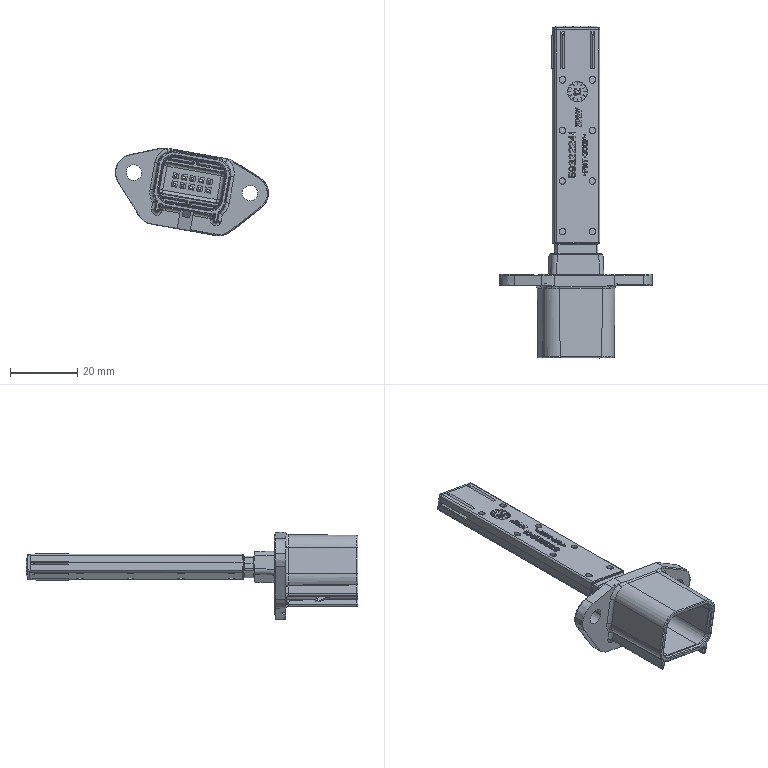Part | SolidWorks | features BaseBody 1 | 1 solid | 1461 faces | box 45.461 x 98.495 x 26.021 mm | volume 9928 mm3 | plane 1049 | cylinder 278 | spline 94 | torus 18 | sphere 14 | cone 8 | commonest cylinder face diameters 0.2 x118 2 x53 0.4 x39 0.5 x12 1 x12 0.6 x11